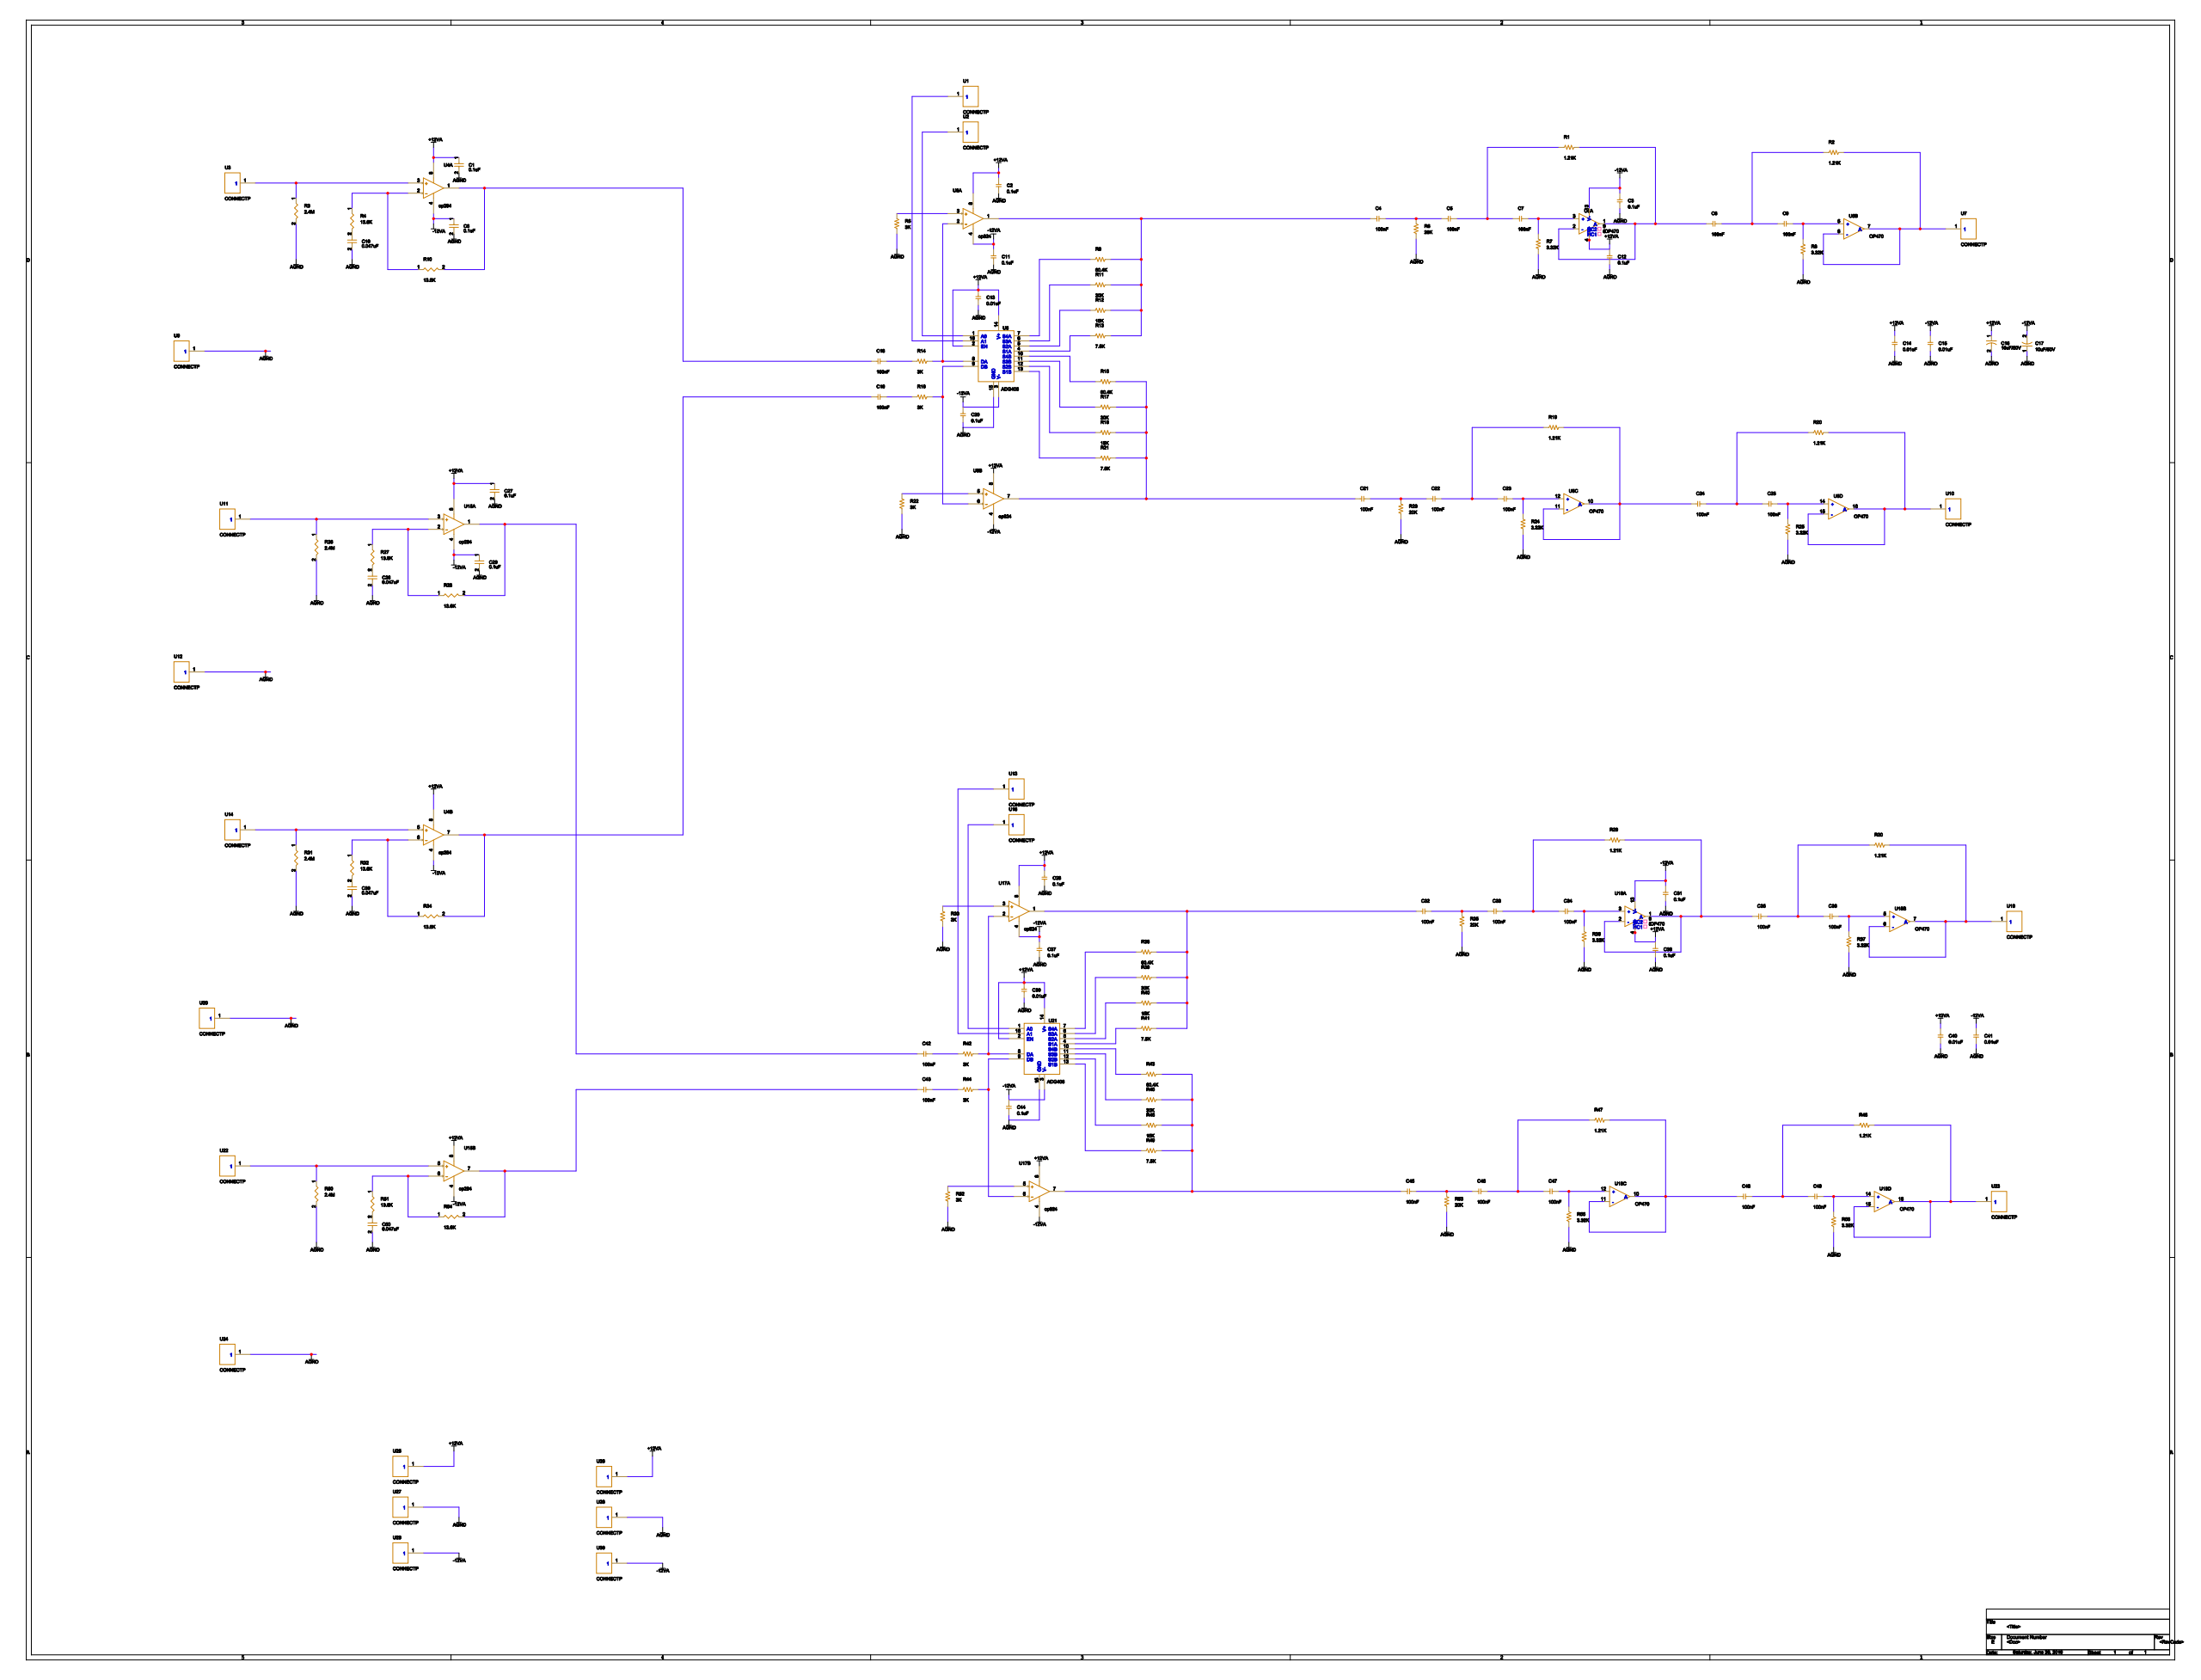Circuit board | Cadence Allegro | 136 parts | 83 nets
Bill of materials:
SYM_NAME,COMP_DEVICE_TYPE,COMP_VALUE,COMP_TOL,COMP_CLASS,REFDES
1206,CAP NP_1_1206_0.1UF,0.1uF,,IC,C1
1206,C_1206_0.1UF,0.1uF,,IC,C2
1206,C_1206_0.1UF,0.1uF,,IC,C3
1206,C_1206_100NF,100nF,,IC,C4
1206,C_1206_100NF,100nF,,IC,C5
1206,CAP NP_1_1206_0.1UF,0.1uF,,IC,C6
1206,C_1206_100NF,100nF,,IC,C7
1206,C_1206_100NF,100nF,,IC,C8
1206,C_1206_100NF,100nF,,IC,C9
1206,CAP NP_1_1206_0.047UF,0.047uF,,IC,C10
1206,C_1206_0.1UF,0.1uF,,IC,C11
1206,C_1206_0.1UF,0.1uF,,IC,C12
1206,C_1206_0.01UF,0.01uF,,IC,C13
1206,C_1206_0.01UF,0.01uF,,IC,C14
1206,C_1206_0.01UF,0.01uF,,IC,C15
7343,CAP_3_7343_10UF/50V,10uF/50V,,IC,C16
7343,CAP_3_7343_10UF/50V,10uF/50V,,IC,C17
1206,C_1206_100NF,100nF,,IC,C18
1206,C_1206_100NF,100nF,,IC,C19
1206,C_1206_0.1UF,0.1uF,,IC,C20
1206,C_1206_100NF,100nF,,IC,C21
1206,C_1206_100NF,100nF,,IC,C22
1206,C_1206_100NF,100nF,,IC,C23
1206,C_1206_100NF,100nF,,IC,C24
1206,C_1206_100NF,100nF,,IC,C25
1206,CAP NP_1_1206_0.047UF,0.047uF,,IC,C26
1206,CAP NP_1_1206_0.1UF,0.1uF,,IC,C27
1206,C_1206_0.1UF,0.1uF,,IC,C28
1206,CAP NP_1_1206_0.1UF,0.1uF,,IC,C29
1206,CAP NP_1_1206_0.047UF,0.047uF,,IC,C30
1206,C_1206_0.1UF,0.1uF,,IC,C31
1206,C_1206_100NF,100nF,,IC,C32
1206,C_1206_100NF,100nF,,IC,C33
1206,C_1206_100NF,100nF,,IC,C34
1206,C_1206_100NF,100nF,,IC,C35
1206,C_1206_100NF,100nF,,IC,C36
1206,C_1206_0.1UF,0.1uF,,IC,C37
1206,C_1206_0.1UF,0.1uF,,IC,C38
1206,C_1206_0.01UF,0.01uF,,IC,C39
1206,C_1206_0.01UF,0.01uF,,IC,C40
1206,C_1206_0.01UF,0.01uF,,IC,C41
1206,C_1206_100NF,100nF,,IC,C42
1206,C_1206_100NF,100nF,,IC,C43
1206,C_1206_0.1UF,0.1uF,,IC,C44
1206,C_1206_100NF,100nF,,IC,C45
1206,C_1206_100NF,100nF,,IC,C46
1206,C_1206_100NF,100nF,,IC,C47
1206,C_1206_100NF,100nF,,IC,C48
1206,C_1206_100NF,100nF,,IC,C49
1206,CAP NP_1_1206_0.047UF,0.047uF,,IC,C50
1206,R_1206_1.21K,1.21K,,IC,R1
1206,R_1206_1.21K,1.21K,,IC,R2
1206,R_2_1206_2.4M,2.4M,,IC,R3
1206,R_2_1206_13.6K,13.6K,,IC,R4
1206,R_1206_3K,3K,,IC,R5
1206,R_1206_20K,20K,,IC,R6
1206,R_1206_3.32K,3.32K,,IC,R7
1206,R_1206_3.32K,3.32K,,IC,R8
1206,R_1206_60.4K,60.4K,,IC,R9
1206,R_2_1206_13.6K,13.6K,,IC,R10
1206,R_1206_30K,30K,,IC,R11
1206,R_1206_15K,15K,,IC,R12
1206,R_1206_7.5K,7.5K,,IC,R13
1206,R_1206_3K,3K,,IC,R14
1206,R_1206_60.4K,60.4K,,IC,R15
1206,R_1206_3K,3K,,IC,R16
1206,R_1206_30K,30K,,IC,R17
1206,R_1206_15K,15K,,IC,R18
1206,R_1206_1.21K,1.21K,,IC,R19
1206,R_1206_1.21K,1.21K,,IC,R20
1206,R_1206_7.5K,7.5K,,IC,R21
1206,R_1206_3K,3K,,IC,R22
1206,R_1206_20K,20K,,IC,R23
1206,R_1206_3.32K,3.32K,,IC,R24
1206,R_1206_3.32K,3.32K,,IC,R25
1206,R_2_1206_2.4M,2.4M,,IC,R26
1206,R_2_1206_13.6K,13.6K,,IC,R27
1206,R_2_1206_13.6K,13.6K,,IC,R28
1206,R_1206_1.21K,1.21K,,IC,R29
1206,R_1206_1.21K,1.21K,,IC,R30
1206,R_2_1206_2.4M,2.4M,,IC,R31
1206,R_2_1206_13.6K,13.6K,,IC,R32
1206,R_1206_3K,3K,,IC,R33
1206,R_2_1206_13.6K,13.6K,,IC,R34
1206,R_1206_20K,20K,,IC,R35
1206,R_1206_3.32K,3.32K,,IC,R36
1206,R_1206_3.32K,3.32K,,IC,R37
1206,R_1206_60.4K,60.4K,,IC,R38
1206,R_1206_30K,30K,,IC,R39
1206,R_1206_15K,15K,,IC,R40
1206,R_1206_7.5K,7.5K,,IC,R41
1206,R_1206_3K,3K,,IC,R42
1206,R_1206_60.4K,60.4K,,IC,R43
1206,R_1206_3K,3K,,IC,R44
1206,R_1206_30K,30K,,IC,R45
1206,R_1206_15K,15K,,IC,R46
1206,R_1206_1.21K,1.21K,,IC,R47
1206,R_1206_1.21K,1.21K,,IC,R48
1206,R_1206_7.5K,7.5K,,IC,R49
1206,R_2_1206_2.4M,2.4M,,IC,R50
1206,R_2_1206_13.6K,13.6K,,IC,R51
1206,R_1206_3K,3K,,IC,R52
1206,R_1206_20K,20K,,IC,R53
1206,R_2_1206_13.6K,13.6K,,IC,R54
1206,R_1206_3.32K,3.32K,,IC,R55
1206,R_1206_3.32K,3.32K,,IC,R56
CPAD80,CONNECTP_CPAD80_CONNECTP,CONNECTP,,IC,U1
CPAD80,CONNECTP_CPAD80_CONNECTP,CONNECTP,,IC,U2
CPAD80,CONNECTP_CPAD80_CONNECTP,CONNECTP,,IC,U3
SO-8,AD8027_2_SO-8_OP284,op284,,IC,U4
SOIC16W,OP470_0_SOIC16W_OP470,OP470,,IC,U5
SO-8,AD8027_2_SO-8_OP824,op824,,IC,U6
CPAD80,CONNECTP_CPAD80_CONNECTP,CONNECTP,,IC,U7
SO-16,ADG406_0_SO-16_ADG406,ADG406,,IC,U8
DP250CIR,CONNECTP_DP250CIR_CONNECTP,CONNECTP,,IC,U9
CPAD80,CONNECTP_CPAD80_CONNECTP,CONNECTP,,IC,U10
CPAD80,CONNECTP_CPAD80_CONNECTP,CONNECTP,,IC,U11
DP250CIR,CONNECTP_DP250CIR_CONNECTP,CONNECTP,,IC,U12
CPAD80,CONNECTP_CPAD80_CONNECTP,CONNECTP,,IC,U13
CPAD80,CONNECTP_CPAD80_CONNECTP,CONNECTP,,IC,U14
SO-8,AD8027_2_SO-8_OP284,op284,,IC,U15
CPAD80,CONNECTP_CPAD80_CONNECTP,CONNECTP,,IC,U16
SO-8,AD8027_2_SO-8_OP824,op824,,IC,U17
SOIC16W,OP470_0_SOIC16W_OP470,OP470,,IC,U18
CPAD80,CONNECTP_CPAD80_CONNECTP,CONNECTP,,IC,U19
DP250CIR,CONNECTP_DP250CIR_CONNECTP,CONNECTP,,IC,U20
SO-16,ADG406_0_SO-16_ADG406,ADG406,,IC,U21
CPAD80,CONNECTP_CPAD80_CONNECTP,CONNECTP,,IC,U22
CPAD80,CONNECTP_CPAD80_CONNECTP,CONNECTP,,IC,U23
DP250CIR,CONNECTP_DP250CIR_CONNECTP,CONNECTP,,IC,U24
CPAD80,CONNECTP_CPAD80_CONNECTP,CONNECTP,,IC,U25
CPAD80,CONNECTP_CPAD80_CONNECTP,CONNECTP,,IC,U26
CPAD80,CONNECTP_CPAD80_CONNECTP,CONNECTP,,IC,U27
CPAD80,CONNECTP_CPAD80_CONNECTP,CONNECTP,,IC,U28
CPAD80,CONNECTP_CPAD80_CONNECTP,CONNECTP,,IC,U29
CPAD80,CONNECTP_CPAD80_CONNECTP,CONNECTP,,IC,U30
Netlist (net: part-pin ...):
N38943: R26-1 U11-1 U15-3
N38967: R27-1 R28-1 U15-2
N38955: C42-2 R28-2 U15-1
+12VA: C1-1 C2-2 C12-2 C13-2 C14-2 C16-1 C27-1 C28-2 C38-2 C39-2 C40-2 U4-8 U5-4 U6-8 U8-2 U8-14 U15-8 U17-8 U18-4 U21-2 U21-14 U25-1 U26-1
-12VA: C3-2 C6-1 C11-2 C15-2 C17-2 C20-2 C29-1 C31-2 C37-2 C41-2 C44-2 U4-4 U5-13 U6-4 U8-3 U15-4 U17-4 U18-13 U21-3 U29-1 U30-1
N39933: R50-1 U15-5 U22-1
N39957: R51-1 R54-1 U15-6
N39945: C43-2 R54-2 U15-7
N38701: R3-1 U3-1 U4-3
N38725: R4-1 R10-1 U4-2
N38713: C18-2 R10-2 U4-1
N39691: R31-1 U4-5 U14-1
N39715: R32-1 R34-1 U4-6
N39703: C19-2 R34-2 U4-7
N65725: R33-2 U17-3
N65945: R42-1 U17-2 U21-8
N65841: C32-2 R38-1 R39-1 R40-1 R41-1 U17-1
N67199: R52-2 U17-5
N66821: R44-1 U17-6 U21-9
N66849: C45-2 R43-1 R45-1 R46-1 R49-1 U17-7
N61503: R5-2 U6-3
N61723: R14-1 U6-2 U8-8
N61619: C4-2 R9-1 R11-1 R12-1 R13-1 U6-1
N62977: R22-2 U6-5
N62599: R16-1 U6-6 U8-9
N62627: C21-2 R15-1 R17-1 R18-1 R21-1 U6-7
N65869: C34-1 R36-2 U18-3
N65549: C35-2 R29-2 U18-1 U18-2
N65993: C36-1 R37-2 U18-5
N65581: R30-2 U18-6 U18-7 U19-1
N67309: C47-1 R55-2 U18-12
N67089: C48-2 R47-2 U18-10 U18-11
N67425: C49-1 R56-2 U18-14
N67133: R48-2 U18-15 U18-16 U23-1
N61647: C7-1 R7-2 U5-3
N61327: C8-2 R1-2 U5-1 U5-2
N61771: C9-1 R8-2 U5-5
N61359: R2-2 U5-6 U5-7 U7-1
N63087: C23-1 R24-2 U5-12
N62867: C24-2 R19-2 U5-10 U5-11
N63203: C25-1 R25-2 U5-14
N62911: R20-2 U5-15 U5-16 U10-1
N65517: U16-1 U21-1
N65495: U13-1 U21-16
AGND: C1-2 C2-1 C3-1 C6-2 C10-2 C11-1 C12-1 C13-1 C14-1 C15-1 C16-2 C17-1 C20-1 C26-2 C27-2 C28-1 C29-2 C30-2 C31-1 C37-1 C38-1 C39-1 C40-1 C41-1 C44-1 C50-2 R3-2 R5-1 R6-1 R7-1 R8-1 R22-1 R23-1 R24-1 R25-1 R26-2 R31-2 R33-1 R35-1 R36-1 R37-1 R50-2 R52-1 R53-1 R55-1 R56-1 U8-15 U9-1 U12-1 U20-1 U21-15 U24-1 U27-1 U28-1
N66633: R41-2 U21-4
N66813: R49-2 U21-13
N66465: R40-2 U21-5
N66797: R46-2 U21-12
N66289: R39-2 U21-6
N66769: R45-2 U21-11
N66197: R38-2 U21-7
N66729: R43-2 U21-10
N61295: U2-1 U8-1
N61273: U1-1 U8-16
N62411: R13-2 U8-4
N62591: R21-2 U8-13
N62243: R12-2 U8-5
N62575: R18-2 U8-12
N62067: R11-2 U8-6
N62547: R17-2 U8-11
N61975: R9-2 U8-7
N62507: R15-2 U8-10
N67293: C45-1 C46-2 R53-2
N65853: C32-1 C33-2 R35-2
N63071: C21-1 C22-2 R23-2
N61631: C4-1 C5-2 R6-2
N66913: C43-1 R44-2
N66745: C42-1 R42-2
N62691: C19-1 R16-2
N62523: C18-1 R14-2
N67125: C48-1 C49-2 R48-1
N67081: C46-1 C47-2 R47-1
N65573: C35-1 C36-2 R30-1
N65541: C33-1 C34-2 R29-1
N62903: C24-1 C25-2 R20-1
N62859: C22-1 C23-2 R19-1
N61351: C8-1 C9-2 R2-1
N61319: C5-1 C7-2 R1-1
N399971: C50-1 R51-2
N397551: C30-1 R32-2
N390071: C26-1 R27-2
N387651: C10-1 R4-2